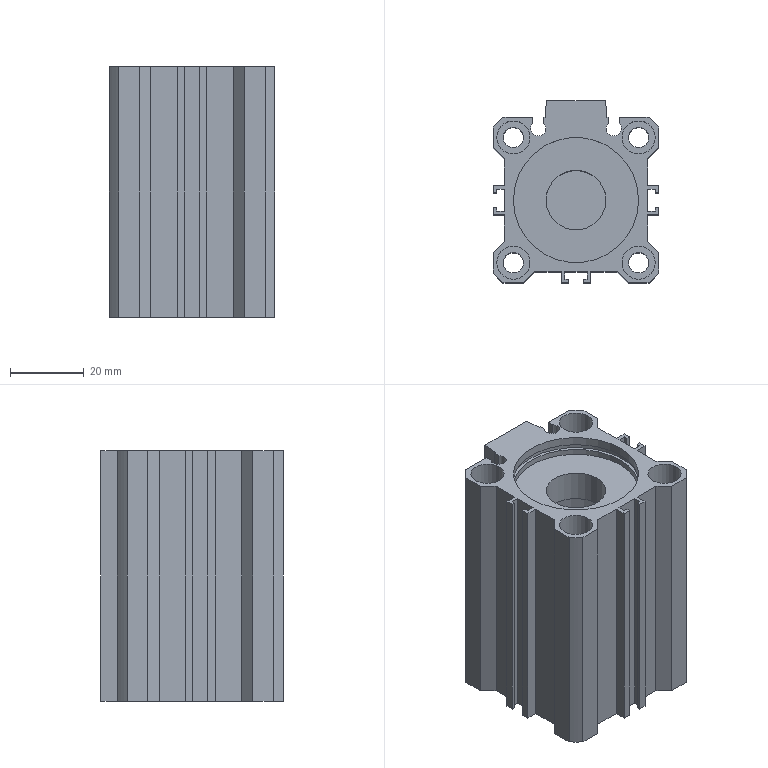Part | NX | features CDQ2B32-35DM_CQ2Tube_32B 2 | 1 solid | 110 faces | box 45 x 49.5 x 68 mm | volume 72766 mm3 | plane 82 | cylinder 28 | commonest cylinder face diameters 9 x8 5.5 x4 60 x4 4.15 x2 9.8 x2 16.25 x2